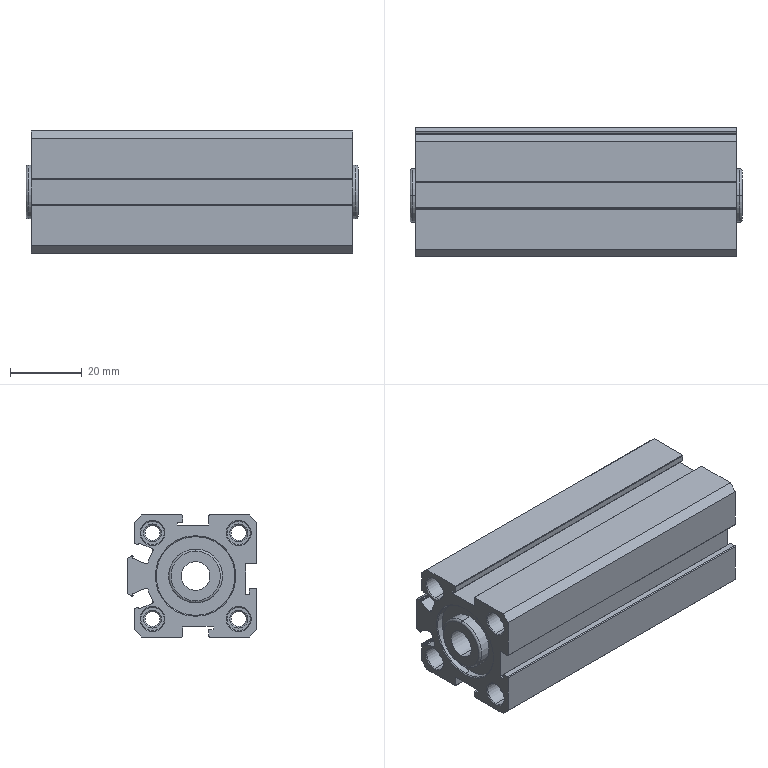Part | STEP file | 001-006-SDAJS_20x60_60b | 1 solid | 208 faces | box 92.5 x 36 x 34 mm | volume 63819 mm3 | cylinder 94 | plane 66 | cone 44 | torus 4 | commonest cylinder face diameters 0.4 x26 4.134 x20 6.5 x16 4.2 x8 0.6 x5 0.8 x5